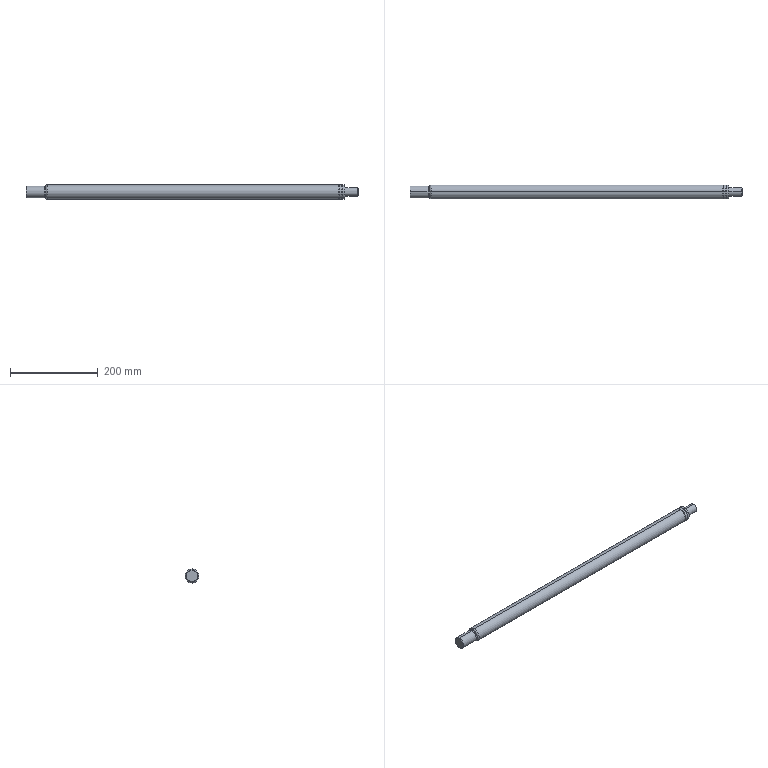Part | SolidWorks | features Revolution 1 | 1 solid | 33 faces | box 755 x 32 x 32 mm | volume 580870 mm3 | cylinder 16 | plane 9 | cone 6 | torus 2 | commonest cylinder face diameters 32 x6 29 x4 20 x2 25 x2 27 x2
STEP:
#1=CARTESIAN_POINT('',(755.,0.,9.));
#2=VERTEX_POINT('',#1);
#3=CARTESIAN_POINT('',(755.,0.,-9.));
#4=VERTEX_POINT('',#3);
#5=CARTESIAN_POINT('',(755.,0.,0.));
#6=DIRECTION('',(-1.,0.,0.));
#7=DIRECTION('',(0.,0.,1.));
#8=AXIS2_PLACEMENT_3D('',#5,#6,#7);
#9=CIRCLE('',#8,9.);
#10=EDGE_CURVE('',#2,#4,#9,.T.);
#11=ORIENTED_EDGE('',*,*,#10,.T.);
#12=CARTESIAN_POINT('',(754.,0.,-10.));
#13=VERTEX_POINT('',#12);
#14=CARTESIAN_POINT('',(755.,0.,-9.));
#15=DIRECTION('',(-0.7071,0.,-0.7071));
#16=VECTOR('',#15,1000.);
#17=LINE('',#14,#16);
#18=EDGE_CURVE('',#4,#13,#17,.T.);
#19=ORIENTED_EDGE('',*,*,#18,.T.);
#20=CARTESIAN_POINT('',(754.,0.,10.));
#21=VERTEX_POINT('',#20);
#22=CARTESIAN_POINT('',(754.,0.,0.));
#23=DIRECTION('',(-1.,0.,0.));
#24=DIRECTION('',(0.,0.,1.));
#25=AXIS2_PLACEMENT_3D('',#22,#23,#24);
#26=CIRCLE('',#25,10.);
#27=EDGE_CURVE('',#21,#13,#26,.T.);
#28=ORIENTED_EDGE('',*,*,#27,.F.);
#29=CARTESIAN_POINT('',(755.,0.,9.));
#30=DIRECTION('',(-0.7071,0.,0.7071));
#31=VECTOR('',#30,1000.);
#32=LINE('',#29,#31);
#33=EDGE_CURVE('',#2,#21,#32,.T.);
#34=ORIENTED_EDGE('',*,*,#33,.F.);
#35=EDGE_LOOP('',(#11,#19,#28,#34));
#36=FACE_OUTER_BOUND('',#35,.T.);
#37=CARTESIAN_POINT('',(755.,0.,0.));
#38=DIRECTION('',(-1.,0.,0.));
#39=DIRECTION('',(0.,0.,1.));
#40=AXIS2_PLACEMENT_3D('',#37,#38,#39);
#41=CONICAL_SURFACE('',#40,9.,0.7854);
#42=ADVANCED_FACE('',(#36),#41,.T.);
#43=ORIENTED_EDGE('',*,*,#27,.T.);
#44=CARTESIAN_POINT('',(725.,0.,-10.));
#45=VERTEX_POINT('',#44);
#46=CARTESIAN_POINT('',(0.,0.,-10.));
#47=DIRECTION('',(-1.,0.,0.));
#48=VECTOR('',#47,1000.);
#49=LINE('',#46,#48);
#50=EDGE_CURVE('',#13,#45,#49,.T.);
#51=ORIENTED_EDGE('',*,*,#50,.T.);
#52=CARTESIAN_POINT('',(725.,0.,10.));
#53=VERTEX_POINT('',#52);
#54=CARTESIAN_POINT('',(725.,0.,0.));
#55=DIRECTION('',(-1.,0.,0.));
#56=DIRECTION('',(0.,0.,1.));
#57=AXIS2_PLACEMENT_3D('',#54,#55,#56);
#58=CIRCLE('',#57,10.);
#59=EDGE_CURVE('',#53,#45,#58,.T.);
#60=ORIENTED_EDGE('',*,*,#59,.F.);
#61=CARTESIAN_POINT('',(0.,0.,10.));
#62=DIRECTION('',(-1.,0.,0.));
#63=VECTOR('',#62,1000.);
#64=LINE('',#61,#63);
#65=EDGE_CURVE('',#21,#53,#64,.T.);
#66=ORIENTED_EDGE('',*,*,#65,.F.);
#67=EDGE_LOOP('',(#43,#51,#60,#66));
#68=FACE_OUTER_BOUND('',#67,.T.);
#69=CARTESIAN_POINT('',(0.,0.,0.));
#70=DIRECTION('',(-1.,0.,0.));
#71=DIRECTION('',(0.,0.,1.));
#72=AXIS2_PLACEMENT_3D('',#69,#70,#71);
#73=CYLINDRICAL_SURFACE('',#72,10.);
#74=ADVANCED_FACE('',(#68),#73,.T.);
#75=CARTESIAN_POINT('',(725.,0.,15.));
#76=VERTEX_POINT('',#75);
#77=CARTESIAN_POINT('',(725.,0.,-15.));
#78=VERTEX_POINT('',#77);
#79=CARTESIAN_POINT('',(725.,0.,0.));
#80=DIRECTION('',(-1.,0.,0.));
#81=DIRECTION('',(0.,0.,1.));
#82=AXIS2_PLACEMENT_3D('',#79,#80,#81);
#83=CIRCLE('',#82,15.);
#84=EDGE_CURVE('',#76,#78,#83,.T.);
#85=ORIENTED_EDGE('',*,*,#84,.T.);
#86=CARTESIAN_POINT('',(724.,0.,-16.));
#87=VERTEX_POINT('',#86);
#88=CARTESIAN_POINT('',(725.,0.,-15.));
#89=DIRECTION('',(-0.7071,0.,-0.7071));
#90=VECTOR('',#89,1000.);
#91=LINE('',#88,#90);
#92=EDGE_CURVE('',#78,#87,#91,.T.);
#93=ORIENTED_EDGE('',*,*,#92,.T.);
#94=CARTESIAN_POINT('',(724.,0.,16.));
#95=VERTEX_POINT('',#94);
#96=CARTESIAN_POINT('',(724.,0.,0.));
#97=DIRECTION('',(-1.,0.,0.));
#98=DIRECTION('',(0.,0.,1.));
#99=AXIS2_PLACEMENT_3D('',#96,#97,#98);
#100=CIRCLE('',#99,16.);
#101=EDGE_CURVE('',#95,#87,#100,.T.);
#102=ORIENTED_EDGE('',*,*,#101,.F.);
#103=CARTESIAN_POINT('',(725.,0.,15.));
#104=DIRECTION('',(-0.7071,0.,0.7071));
#105=VECTOR('',#104,1000.);
#106=LINE('',#103,#105);
#107=EDGE_CURVE('',#76,#95,#106,.T.);
#108=ORIENTED_EDGE('',*,*,#107,.F.);
#109=EDGE_LOOP('',(#85,#93,#102,#108));
#110=FACE_OUTER_BOUND('',#109,.T.);
#111=CARTESIAN_POINT('',(725.,0.,0.));
#112=DIRECTION('',(-1.,0.,0.));
#113=DIRECTION('',(0.,0.,1.));
#114=AXIS2_PLACEMENT_3D('',#111,#112,#113);
#115=CONICAL_SURFACE('',#114,15.,0.7854);
#116=ADVANCED_FACE('',(#110),#115,.T.);
#117=ORIENTED_EDGE('',*,*,#101,.T.);
#118=CARTESIAN_POINT('',(720.,0.,-16.));
#119=VERTEX_POINT('',#118);
#120=CARTESIAN_POINT('',(0.,0.,-16.));
#121=DIRECTION('',(-1.,0.,0.));
#122=VECTOR('',#121,1000.);
#123=LINE('',#120,#122);
#124=EDGE_CURVE('',#87,#119,#123,.T.);
#125=ORIENTED_EDGE('',*,*,#124,.T.);
#126=CARTESIAN_POINT('',(720.,0.,16.));
#127=VERTEX_POINT('',#126);
#128=CARTESIAN_POINT('',(720.,0.,0.));
#129=DIRECTION('',(-1.,0.,0.));
#130=DIRECTION('',(0.,0.,1.));
#131=AXIS2_PLACEMENT_3D('',#128,#129,#130);
#132=CIRCLE('',#131,16.);
#133=EDGE_CURVE('',#127,#119,#132,.T.);
#134=ORIENTED_EDGE('',*,*,#133,.F.);
#135=CARTESIAN_POINT('',(0.,0.,16.));
#136=DIRECTION('',(-1.,0.,0.));
#137=VECTOR('',#136,1000.);
#138=LINE('',#135,#137);
#139=EDGE_CURVE('',#95,#127,#138,.T.);
#140=ORIENTED_EDGE('',*,*,#139,.F.);
#141=EDGE_LOOP('',(#117,#125,#134,#140));
#142=FACE_OUTER_BOUND('',#141,.T.);
#143=CARTESIAN_POINT('',(0.,0.,0.));
#144=DIRECTION('',(-1.,0.,0.));
#145=DIRECTION('',(0.,0.,1.));
#146=AXIS2_PLACEMENT_3D('',#143,#144,#145);
#147=CYLINDRICAL_SURFACE('',#146,16.);
#148=ADVANCED_FACE('',(#142),#147,.T.);
#149=CARTESIAN_POINT('',(720.,0.,14.5));
#150=VERTEX_POINT('',#149);
#151=CARTESIAN_POINT('',(720.,0.,-14.5));
#152=VERTEX_POINT('',#151);
#153=CARTESIAN_POINT('',(720.,0.,0.));
#154=DIRECTION('',(-1.,0.,0.));
#155=DIRECTION('',(0.,0.,1.));
#156=AXIS2_PLACEMENT_3D('',#153,#154,#155);
#157=CIRCLE('',#156,14.5);
#158=EDGE_CURVE('',#150,#152,#157,.T.);
#159=ORIENTED_EDGE('',*,*,#158,.T.);
#160=CARTESIAN_POINT('',(718.,0.,-14.5));
#161=VERTEX_POINT('',#160);
#162=CARTESIAN_POINT('',(0.,0.,-14.5));
#163=DIRECTION('',(-1.,0.,0.));
#164=VECTOR('',#163,1000.);
#165=LINE('',#162,#164);
#166=EDGE_CURVE('',#152,#161,#165,.T.);
#167=ORIENTED_EDGE('',*,*,#166,.T.);
#168=CARTESIAN_POINT('',(718.,0.,14.5));
#169=VERTEX_POINT('',#168);
#170=CARTESIAN_POINT('',(718.,0.,0.));
#171=DIRECTION('',(-1.,0.,0.));
#172=DIRECTION('',(0.,0.,1.));
#173=AXIS2_PLACEMENT_3D('',#170,#171,#172);
#174=CIRCLE('',#173,14.5);
#175=EDGE_CURVE('',#169,#161,#174,.T.);
#176=ORIENTED_EDGE('',*,*,#175,.F.);
#177=CARTESIAN_POINT('',(0.,0.,14.5));
#178=DIRECTION('',(-1.,0.,0.));
#179=VECTOR('',#178,1000.);
#180=LINE('',#177,#179);
#181=EDGE_CURVE('',#150,#169,#180,.T.);
#182=ORIENTED_EDGE('',*,*,#181,.F.);
#183=EDGE_LOOP('',(#159,#167,#176,#182));
#184=FACE_OUTER_BOUND('',#183,.T.);
#185=CARTESIAN_POINT('',(0.,0.,0.));
#186=DIRECTION('',(-1.,0.,0.));
#187=DIRECTION('',(0.,0.,1.));
#188=AXIS2_PLACEMENT_3D('',#185,#186,#187);
#189=CYLINDRICAL_SURFACE('',#188,14.5);
#190=ADVANCED_FACE('',(#184),#189,.T.);
#191=CARTESIAN_POINT('',(718.,0.,16.));
#192=VERTEX_POINT('',#191);
#193=CARTESIAN_POINT('',(718.,0.,-16.));
#194=VERTEX_POINT('',#193);
#195=CARTESIAN_POINT('',(718.,0.,0.));
#196=DIRECTION('',(-1.,0.,0.));
#197=DIRECTION('',(0.,0.,1.));
#198=AXIS2_PLACEMENT_3D('',#195,#196,#197);
#199=CIRCLE('',#198,16.);
#200=EDGE_CURVE('',#192,#194,#199,.T.);
#201=ORIENTED_EDGE('',*,*,#200,.T.);
#202=CARTESIAN_POINT('',(713.,0.,-16.));
#203=VERTEX_POINT('',#202);
#204=CARTESIAN_POINT('',(0.,0.,-16.));
#205=DIRECTION('',(-1.,0.,0.));
#206=VECTOR('',#205,1000.);
#207=LINE('',#204,#206);
#208=EDGE_CURVE('',#194,#203,#207,.T.);
#209=ORIENTED_EDGE('',*,*,#208,.T.);
#210=CARTESIAN_POINT('',(713.,0.,16.));
#211=VERTEX_POINT('',#210);
#212=CARTESIAN_POINT('',(713.,0.,0.));
#213=DIRECTION('',(-1.,0.,0.));
#214=DIRECTION('',(0.,0.,1.));
#215=AXIS2_PLACEMENT_3D('',#212,#213,#214);
#216=CIRCLE('',#215,16.);
#217=EDGE_CURVE('',#211,#203,#216,.T.);
#218=ORIENTED_EDGE('',*,*,#217,.F.);
#219=CARTESIAN_POINT('',(0.,0.,16.));
#220=DIRECTION('',(-1.,0.,0.));
#221=VECTOR('',#220,1000.);
#222=LINE('',#219,#221);
#223=EDGE_CURVE('',#192,#211,#222,.T.);
#224=ORIENTED_EDGE('',*,*,#223,.F.);
#225=EDGE_LOOP('',(#201,#209,#218,#224));
#226=FACE_OUTER_BOUND('',#225,.T.);
#227=CARTESIAN_POINT('',(0.,0.,0.));
#228=DIRECTION('',(-1.,0.,0.));
#229=DIRECTION('',(0.,0.,1.));
#230=AXIS2_PLACEMENT_3D('',#227,#228,#229);
#231=CYLINDRICAL_SURFACE('',#230,16.);
#232=ADVANCED_FACE('',(#226),#231,.T.);
#233=CARTESIAN_POINT('',(713.,0.,14.5));
#234=VERTEX_POINT('',#233);
#235=CARTESIAN_POINT('',(713.,0.,-14.5));
#236=VERTEX_POINT('',#235);
#237=CARTESIAN_POINT('',(713.,0.,0.));
#238=DIRECTION('',(-1.,0.,0.));
#239=DIRECTION('',(0.,0.,1.));
#240=AXIS2_PLACEMENT_3D('',#237,#238,#239);
#241=CIRCLE('',#240,14.5);
#242=EDGE_CURVE('',#234,#236,#241,.T.);
#243=ORIENTED_EDGE('',*,*,#242,.T.);
#244=CARTESIAN_POINT('',(711.,0.,-14.5));
#245=VERTEX_POINT('',#244);
#246=CARTESIAN_POINT('',(0.,0.,-14.5));
#247=DIRECTION('',(-1.,0.,0.));
#248=VECTOR('',#247,1000.);
#249=LINE('',#246,#248);
#250=EDGE_CURVE('',#236,#245,#249,.T.);
#251=ORIENTED_EDGE('',*,*,#250,.T.);
#252=CARTESIAN_POINT('',(711.,0.,14.5));
#253=VERTEX_POINT('',#252);
#254=CARTESIAN_POINT('',(711.,0.,0.));
#255=DIRECTION('',(-1.,0.,0.));
#256=DIRECTION('',(0.,0.,1.));
#257=AXIS2_PLACEMENT_3D('',#254,#255,#256);
#258=CIRCLE('',#257,14.5);
#259=EDGE_CURVE('',#253,#245,#258,.T.);
#260=ORIENTED_EDGE('',*,*,#259,.F.);
#261=CARTESIAN_POINT('',(0.,0.,14.5));
#262=DIRECTION('',(-1.,0.,0.));
#263=VECTOR('',#262,1000.);
#264=LINE('',#261,#263);
#265=EDGE_CURVE('',#234,#253,#264,.T.);
#266=ORIENTED_EDGE('',*,*,#265,.F.);
#267=EDGE_LOOP('',(#243,#251,#260,#266));
#268=FACE_OUTER_BOUND('',#267,.T.);
#269=CARTESIAN_POINT('',(0.,0.,0.));
#270=DIRECTION('',(-1.,0.,0.));
#271=DIRECTION('',(0.,0.,1.));
#272=AXIS2_PLACEMENT_3D('',#269,#270,#271);
#273=CYLINDRICAL_SURFACE('',#272,14.5);
#274=ADVANCED_FACE('',(#268),#273,.T.);
#275=CARTESIAN_POINT('',(711.,0.,16.));
#276=VERTEX_POINT('',#275);
#277=CARTESIAN_POINT('',(711.,0.,-16.));
#278=VERTEX_POINT('',#277);
#279=CARTESIAN_POINT('',(711.,0.,0.));
#280=DIRECTION('',(-1.,0.,0.));
#281=DIRECTION('',(0.,0.,1.));
#282=AXIS2_PLACEMENT_3D('',#279,#280,#281);
#283=CIRCLE('',#282,16.);
#284=EDGE_CURVE('',#276,#278,#283,.T.);
#285=ORIENTED_EDGE('',*,*,#284,.T.);
#286=CARTESIAN_POINT('',(48.,0.,-16.));
#287=VERTEX_POINT('',#286);
#288=CARTESIAN_POINT('',(0.,0.,-16.));
#289=DIRECTION('',(-1.,0.,0.));
#290=VECTOR('',#289,1000.);
#291=LINE('',#288,#290);
#292=EDGE_CURVE('',#278,#287,#291,.T.);
#293=ORIENTED_EDGE('',*,*,#292,.T.);
#294=CARTESIAN_POINT('',(48.,0.,16.));
#295=VERTEX_POINT('',#294);
#296=CARTESIAN_POINT('',(48.,0.,0.));
#297=DIRECTION('',(-1.,0.,0.));
#298=DIRECTION('',(0.,0.,1.));
#299=AXIS2_PLACEMENT_3D('',#296,#297,#298);
#300=CIRCLE('',#299,16.);
#301=EDGE_CURVE('',#295,#287,#300,.T.);
#302=ORIENTED_EDGE('',*,*,#301,.F.);
#303=CARTESIAN_POINT('',(0.,0.,16.));
#304=DIRECTION('',(-1.,0.,0.));
#305=VECTOR('',#304,1000.);
#306=LINE('',#303,#305);
#307=EDGE_CURVE('',#276,#295,#306,.T.);
#308=ORIENTED_EDGE('',*,*,#307,.F.);
#309=EDGE_LOOP('',(#285,#293,#302,#308));
#310=FACE_OUTER_BOUND('',#309,.T.);
#311=CARTESIAN_POINT('',(0.,0.,0.));
#312=DIRECTION('',(-1.,0.,0.));
#313=DIRECTION('',(0.,0.,1.));
#314=AXIS2_PLACEMENT_3D('',#311,#312,#313);
#315=CYLINDRICAL_SURFACE('',#314,16.);
#316=ADVANCED_FACE('',(#310),#315,.T.);
#317=ORIENTED_EDGE('',*,*,#301,.T.);
#318=CARTESIAN_POINT('',(45.,0.,-13.));
#319=VERTEX_POINT('',#318);
#320=CARTESIAN_POINT('',(48.,0.,-13.));
#321=DIRECTION('',(0.,1.,0.));
#322=DIRECTION('',(0.,0.,1.));
#323=AXIS2_PLACEMENT_3D('',#320,#321,#322);
#324=CIRCLE('',#323,3.);
#325=EDGE_CURVE('',#287,#319,#324,.T.);
#326=ORIENTED_EDGE('',*,*,#325,.T.);
#327=CARTESIAN_POINT('',(45.,0.,13.));
#328=VERTEX_POINT('',#327);
#329=CARTESIAN_POINT('',(45.,0.,0.));
#330=DIRECTION('',(-1.,0.,0.));
#331=DIRECTION('',(0.,0.,1.));
#332=AXIS2_PLACEMENT_3D('',#329,#330,#331);
#333=CIRCLE('',#332,13.);
#334=EDGE_CURVE('',#328,#319,#333,.T.);
#335=ORIENTED_EDGE('',*,*,#334,.F.);
#336=CARTESIAN_POINT('',(48.,0.,13.));
#337=DIRECTION('',(0.,-1.,0.));
#338=DIRECTION('',(0.,0.,-1.));
#339=AXIS2_PLACEMENT_3D('',#336,#337,#338);
#340=CIRCLE('',#339,3.);
#341=EDGE_CURVE('',#295,#328,#340,.T.);
#342=ORIENTED_EDGE('',*,*,#341,.F.);
#343=EDGE_LOOP('',(#317,#326,#335,#342));
#344=FACE_OUTER_BOUND('',#343,.T.);
#345=CARTESIAN_POINT('',(48.,0.,0.));
#346=DIRECTION('',(-1.,0.,0.));
#347=DIRECTION('',(0.,0.,1.));
#348=AXIS2_PLACEMENT_3D('',#345,#346,#347);
#349=TOROIDAL_SURFACE('',#348,13.,3.);
#350=ADVANCED_FACE('',(#344),#349,.T.);
#351=CARTESIAN_POINT('',(45.,0.,12.5));
#352=VERTEX_POINT('',#351);
#353=CARTESIAN_POINT('',(45.,0.,-12.5));
#354=VERTEX_POINT('',#353);
#355=CARTESIAN_POINT('',(45.,0.,0.));
#356=DIRECTION('',(-1.,0.,0.));
#357=DIRECTION('',(0.,0.,1.));
#358=AXIS2_PLACEMENT_3D('',#355,#356,#357);
#359=CIRCLE('',#358,12.5);
#360=EDGE_CURVE('',#352,#354,#359,.T.);
#361=ORIENTED_EDGE('',*,*,#360,.T.);
#362=CARTESIAN_POINT('',(41.,0.,-12.5));
#363=VERTEX_POINT('',#362);
#364=CARTESIAN_POINT('',(0.,0.,-12.5));
#365=DIRECTION('',(-1.,0.,0.));
#366=VECTOR('',#365,1000.);
#367=LINE('',#364,#366);
#368=EDGE_CURVE('',#354,#363,#367,.T.);
#369=ORIENTED_EDGE('',*,*,#368,.T.);
#370=CARTESIAN_POINT('',(41.,0.,12.5));
#371=VERTEX_POINT('',#370);
#372=CARTESIAN_POINT('',(41.,0.,0.));
#373=DIRECTION('',(-1.,0.,0.));
#374=DIRECTION('',(0.,0.,1.));
#375=AXIS2_PLACEMENT_3D('',#372,#373,#374);
#376=CIRCLE('',#375,12.5);
#377=EDGE_CURVE('',#371,#363,#376,.T.);
#378=ORIENTED_EDGE('',*,*,#377,.F.);
#379=CARTESIAN_POINT('',(0.,0.,12.5));
#380=DIRECTION('',(-1.,0.,0.));
#381=VECTOR('',#380,1000.);
#382=LINE('',#379,#381);
#383=EDGE_CURVE('',#352,#371,#382,.T.);
#384=ORIENTED_EDGE('',*,*,#383,.F.);
#385=EDGE_LOOP('',(#361,#369,#378,#384));
#386=FACE_OUTER_BOUND('',#385,.T.);
#387=CARTESIAN_POINT('',(0.,0.,0.));
#388=DIRECTION('',(-1.,0.,0.));
#389=DIRECTION('',(0.,0.,1.));
#390=AXIS2_PLACEMENT_3D('',#387,#388,#389);
#391=CYLINDRICAL_SURFACE('',#390,12.5);
#392=ADVANCED_FACE('',(#386),#391,.T.);
#393=CARTESIAN_POINT('',(41.,0.,13.5));
#394=VERTEX_POINT('',#393);
#395=CARTESIAN_POINT('',(41.,0.,-13.5));
#396=VERTEX_POINT('',#395);
#397=CARTESIAN_POINT('',(41.,0.,0.));
#398=DIRECTION('',(-1.,0.,0.));
#399=DIRECTION('',(0.,0.,1.));
#400=AXIS2_PLACEMENT_3D('',#397,#398,#399);
#401=CIRCLE('',#400,13.5);
#402=EDGE_CURVE('',#394,#396,#401,.T.);
#403=ORIENTED_EDGE('',*,*,#402,.T.);
#404=CARTESIAN_POINT('',(1.,0.,-13.5));
#405=VERTEX_POINT('',#404);
#406=CARTESIAN_POINT('',(0.,0.,-13.5));
#407=DIRECTION('',(-1.,0.,0.));
#408=VECTOR('',#407,1000.);
#409=LINE('',#406,#408);
#410=EDGE_CURVE('',#396,#405,#409,.T.);
#411=ORIENTED_EDGE('',*,*,#410,.T.);
#412=CARTESIAN_POINT('',(1.,0.,13.5));
#413=VERTEX_POINT('',#412);
#414=CARTESIAN_POINT('',(1.,0.,0.));
#415=DIRECTION('',(-1.,0.,0.));
#416=DIRECTION('',(0.,0.,1.));
#417=AXIS2_PLACEMENT_3D('',#414,#415,#416);
#418=CIRCLE('',#417,13.5);
#419=EDGE_CURVE('',#413,#405,#418,.T.);
#420=ORIENTED_EDGE('',*,*,#419,.F.);
#421=CARTESIAN_POINT('',(0.,0.,13.5));
#422=DIRECTION('',(-1.,0.,0.));
#423=VECTOR('',#422,1000.);
#424=LINE('',#421,#423);
#425=EDGE_CURVE('',#394,#413,#424,.T.);
#426=ORIENTED_EDGE('',*,*,#425,.F.);
#427=EDGE_LOOP('',(#403,#411,#420,#426));
#428=FACE_OUTER_BOUND('',#427,.T.);
#429=CARTESIAN_POINT('',(0.,0.,0.));
#430=DIRECTION('',(-1.,0.,0.));
#431=DIRECTION('',(0.,0.,1.));
#432=AXIS2_PLACEMENT_3D('',#429,#430,#431);
#433=CYLINDRICAL_SURFACE('',#432,13.5);
#434=ADVANCED_FACE('',(#428),#433,.T.);
#435=CARTESIAN_POINT('',(0.,0.,12.5));
#436=VERTEX_POINT('',#435);
#437=CARTESIAN_POINT('',(0.,0.,-12.5));
#438=VERTEX_POINT('',#437);
#439=CARTESIAN_POINT('',(0.,0.,0.));
#440=DIRECTION('',(-1.,0.,0.));
#441=DIRECTION('',(0.,0.,1.));
#442=AXIS2_PLACEMENT_3D('',#439,#440,#441);
#443=CIRCLE('',#442,12.5);
#444=EDGE_CURVE('',#436,#438,#443,.T.);
#445=ORIENTED_EDGE('',*,*,#444,.F.);
#446=CARTESIAN_POINT('',(1.,0.,13.5));
#447=DIRECTION('',(0.7071,0.,0.7071));
#448=VECTOR('',#447,1000.);
#449=LINE('',#446,#448);
#450=EDGE_CURVE('',#436,#413,#449,.T.);
#451=ORIENTED_EDGE('',*,*,#450,.T.);
#452=ORIENTED_EDGE('',*,*,#419,.T.);
#453=CARTESIAN_POINT('',(1.,0.,-13.5));
#454=DIRECTION('',(0.7071,0.,-0.7071));
#455=VECTOR('',#454,1000.);
#456=LINE('',#453,#455);
#457=EDGE_CURVE('',#438,#405,#456,.T.);
#458=ORIENTED_EDGE('',*,*,#457,.F.);
#459=EDGE_LOOP('',(#445,#451,#452,#458));
#460=FACE_OUTER_BOUND('',#459,.T.);
#461=CARTESIAN_POINT('',(1.,0.,0.));
#462=DIRECTION('',(1.,0.,0.));
#463=DIRECTION('',(0.,0.,-1.));
#464=AXIS2_PLACEMENT_3D('',#461,#462,#463);
#465=CONICAL_SURFACE('',#464,13.5,0.7854);
#466=ADVANCED_FACE('',(#460),#465,.T.);
#467=CARTESIAN_POINT('',(0.,0.,0.));
#468=DIRECTION('',(-1.,0.,0.));
#469=DIRECTION('',(0.,0.,1.));
#470=AXIS2_PLACEMENT_3D('',#467,#468,#469);
#471=CIRCLE('',#470,12.5);
#472=EDGE_CURVE('',#438,#436,#471,.T.);
#473=ORIENTED_EDGE('',*,*,#472,.T.);
#474=ORIENTED_EDGE('',*,*,#444,.T.);
#475=EDGE_LOOP('',(#473,#474));
#476=FACE_OUTER_BOUND('',#475,.T.);
#477=CARTESIAN_POINT('',(0.,0.,0.));
#478=DIRECTION('',(1.,0.,0.));
#479=DIRECTION('',(0.,0.,-1.));
#480=AXIS2_PLACEMENT_3D('',#477,#478,#479);
#481=PLANE('',#480);
#482=ADVANCED_FACE('',(#476),#481,.F.);
#483=ORIENTED_EDGE('',*,*,#450,.F.);
#484=ORIENTED_EDGE('',*,*,#472,.F.);
#485=ORIENTED_EDGE('',*,*,#457,.T.);
#486=CARTESIAN_POINT('',(1.,0.,0.));
#487=DIRECTION('',(-1.,0.,0.));
#488=DIRECTION('',(0.,0.,1.));
#489=AXIS2_PLACEMENT_3D('',#486,#487,#488);
#490=CIRCLE('',#489,13.5);
#491=EDGE_CURVE('',#405,#413,#490,.T.);
#492=ORIENTED_EDGE('',*,*,#491,.T.);
#493=EDGE_LOOP('',(#483,#484,#485,#492));
#494=FACE_OUTER_BOUND('',#493,.T.);
#495=CARTESIAN_POINT('',(1.,0.,0.));
#496=DIRECTION('',(1.,0.,0.));
#497=DIRECTION('',(0.,0.,-1.));
#498=AXIS2_PLACEMENT_3D('',#495,#496,#497);
#499=CONICAL_SURFACE('',#498,13.5,0.7854);
#500=ADVANCED_FACE('',(#494),#499,.T.);
#501=ORIENTED_EDGE('',*,*,#410,.F.);
#502=CARTESIAN_POINT('',(41.,0.,0.));
#503=DIRECTION('',(-1.,0.,0.));
#504=DIRECTION('',(0.,0.,1.));
#505=AXIS2_PLACEMENT_3D('',#502,#503,#504);
#506=CIRCLE('',#505,13.5);
#507=EDGE_CURVE('',#396,#394,#506,.T.);
#508=ORIENTED_EDGE('',*,*,#507,.T.);
#509=ORIENTED_EDGE('',*,*,#425,.T.);
#510=ORIENTED_EDGE('',*,*,#491,.F.);
#511=EDGE_LOOP('',(#501,#508,#509,#510));
#512=FACE_OUTER_BOUND('',#511,.T.);
#513=CARTESIAN_POINT('',(0.,0.,0.));
#514=DIRECTION('',(-1.,0.,0.));
#515=DIRECTION('',(0.,0.,1.));
#516=AXIS2_PLACEMENT_3D('',#513,#514,#515);
#517=CYLINDRICAL_SURFACE('',#516,13.5);
#518=ADVANCED_FACE('',(#512),#517,.T.);
#519=ORIENTED_EDGE('',*,*,#402,.F.);
#520=ORIENTED_EDGE('',*,*,#507,.F.);
#521=EDGE_LOOP('',(#519,#520));
#522=FACE_OUTER_BOUND('',#521,.T.);
#523=ORIENTED_EDGE('',*,*,#377,.T.);
#524=CARTESIAN_POINT('',(41.,0.,0.));
#525=DIRECTION('',(-1.,0.,0.));
#526=DIRECTION('',(0.,0.,1.));
#527=AXIS2_PLACEMENT_3D('',#524,#525,#526);
#528=CIRCLE('',#527,12.5);
#529=EDGE_CURVE('',#363,#371,#528,.T.);
#530=ORIENTED_EDGE('',*,*,#529,.T.);
#531=EDGE_LOOP('',(#523,#530));
#532=FACE_BOUND('',#531,.T.);
#533=CARTESIAN_POINT('',(41.,13.5,0.));
#534=DIRECTION('',(-1.,0.,0.));
#535=DIRECTION('',(0.,0.,1.));
#536=AXIS2_PLACEMENT_3D('',#533,#534,#535);
#537=PLANE('',#536);
#538=ADVANCED_FACE('',(#522,#532),#537,.F.);
#539=ORIENTED_EDGE('',*,*,#368,.F.);
#540=CARTESIAN_POINT('',(45.,0.,0.));
#541=DIRECTION('',(-1.,0.,0.));
#542=DIRECTION('',(0.,0.,1.));
#543=AXIS2_PLACEMENT_3D('',#540,#541,#542);
#544=CIRCLE('',#543,12.5);
#545=EDGE_CURVE('',#354,#352,#544,.T.);
#546=ORIENTED_EDGE('',*,*,#545,.T.);
#547=ORIENTED_EDGE('',*,*,#383,.T.);
#548=ORIENTED_EDGE('',*,*,#529,.F.);
#549=EDGE_LOOP('',(#539,#546,#547,#548));
#550=FACE_OUTER_BOUND('',#549,.T.);
#551=CARTESIAN_POINT('',(0.,0.,0.));
#552=DIRECTION('',(-1.,0.,0.));
#553=DIRECTION('',(0.,0.,1.));
#554=AXIS2_PLACEMENT_3D('',#551,#552,#553);
#555=CYLINDRICAL_SURFACE('',#554,12.5);
#556=ADVANCED_FACE('',(#550),#555,.T.);
#557=ORIENTED_EDGE('',*,*,#360,.F.);
#558=ORIENTED_EDGE('',*,*,#545,.F.);
#559=EDGE_LOOP('',(#557,#558));
#560=FACE_BOUND('',#559,.T.);
#561=ORIENTED_EDGE('',*,*,#334,.T.);
#562=CARTESIAN_POINT('',(45.,0.,0.));
#563=DIRECTION('',(-1.,0.,0.));
#564=DIRECTION('',(0.,0.,1.));
#565=AXIS2_PLACEMENT_3D('',#562,#563,#564);
#566=CIRCLE('',#565,13.);
#567=EDGE_CURVE('',#319,#328,#566,.T.);
#568=ORIENTED_EDGE('',*,*,#567,.T.);
#569=EDGE_LOOP('',(#561,#568));
#570=FACE_OUTER_BOUND('',#569,.T.);
#571=CARTESIAN_POINT('',(45.,12.5,0.));
#572=DIRECTION('',(1.,0.,0.));
#573=DIRECTION('',(0.,0.,-1.));
#574=AXIS2_PLACEMENT_3D('',#571,#572,#573);
#575=PLANE('',#574);
#576=ADVANCED_FACE('',(#560,#570),#575,.F.);
#577=ORIENTED_EDGE('',*,*,#325,.F.);
#578=CARTESIAN_POINT('',(48.,0.,0.));
#579=DIRECTION('',(-1.,0.,0.));
#580=DIRECTION('',(0.,0.,1.));
#581=AXIS2_PLACEMENT_3D('',#578,#579,#580);
#582=CIRCLE('',#581,16.);
#583=EDGE_CURVE('',#287,#295,#582,.T.);
#584=ORIENTED_EDGE('',*,*,#583,.T.);
#585=ORIENTED_EDGE('',*,*,#341,.T.);
#586=ORIENTED_EDGE('',*,*,#567,.F.);
#587=EDGE_LOOP('',(#577,#584,#585,#586));
#588=FACE_OUTER_BOUND('',#587,.T.);
#589=CARTESIAN_POINT('',(48.,0.,0.));
#590=DIRECTION('',(-1.,0.,0.));
#591=DIRECTION('',(0.,0.,1.));
#592=AXIS2_PLACEMENT_3D('',#589,#590,#591);
#593=TOROIDAL_SURFACE('',#592,13.,3.);
#594=ADVANCED_FACE('',(#588),#593,.T.);
#595=ORIENTED_EDGE('',*,*,#292,.F.);
#596=CARTESIAN_POINT('',(711.,0.,0.));
#597=DIRECTION('',(-1.,0.,0.));
#598=DIRECTION('',(0.,0.,1.));
#599=AXIS2_PLACEMENT_3D('',#596,#597,#598);
#600=CIRCLE('',#599,16.);
#601=EDGE_CURVE('',#278,#276,#600,.T.);
#602=ORIENTED_EDGE('',*,*,#601,.T.);
#603=ORIENTED_EDGE('',*,*,#307,.T.);
#604=ORIENTED_EDGE('',*,*,#583,.F.);
#605=EDGE_LOOP('',(#595,#602,#603,#604));
#606=FACE_OUTER_BOUND('',#605,.T.);
#607=CARTESIAN_POINT('',(0.,0.,0.));
#608=DIRECTION('',(-1.,0.,0.));
#609=DIRECTION('',(0.,0.,1.));
#610=AXIS2_PLACEMENT_3D('',#607,#608,#609);
#611=CYLINDRICAL_SURFACE('',#610,16.);
#612=ADVANCED_FACE('',(#606),#611,.T.);
#613=ORIENTED_EDGE('',*,*,#284,.F.);
#614=ORIENTED_EDGE('',*,*,#601,.F.);
#615=EDGE_LOOP('',(#613,#614));
#616=FACE_OUTER_BOUND('',#615,.T.);
#617=ORIENTED_EDGE('',*,*,#259,.T.);
#618=CARTESIAN_POINT('',(711.,0.,0.));
#619=DIRECTION('',(-1.,0.,0.));
#620=DIRECTION('',(0.,0.,1.));
#621=AXIS2_PLACEMENT_3D('',#618,#619,#620);
#622=CIRCLE('',#621,14.5);
#623=EDGE_CURVE('',#245,#253,#622,.T.);
#624=ORIENTED_EDGE('',*,*,#623,.T.);
#625=EDGE_LOOP('',(#617,#624));
#626=FACE_BOUND('',#625,.T.);
#627=CARTESIAN_POINT('',(711.,16.,0.));
#628=DIRECTION('',(-1.,0.,0.));
#629=DIRECTION('',(0.,0.,1.));
#630=AXIS2_PLACEMENT_3D('',#627,#628,#629);
#631=PLANE('',#630);
#632=ADVANCED_FACE('',(#616,#626),#631,.F.);
#633=ORIENTED_EDGE('',*,*,#250,.F.);
#634=CARTESIAN_POINT('',(713.,0.,0.));
#635=DIRECTION('',(-1.,0.,0.));
#636=DIRECTION('',(0.,0.,1.));
#637=AXIS2_PLACEMENT_3D('',#634,#635,#636);
#638=CIRCLE('',#637,14.5);
#639=EDGE_CURVE('',#236,#234,#638,.T.);
#640=ORIENTED_EDGE('',*,*,#639,.T.);
#641=ORIENTED_EDGE('',*,*,#265,.T.);
#642=ORIENTED_EDGE('',*,*,#623,.F.);
#643=EDGE_LOOP('',(#633,#640,#641,#642));
#644=FACE_OUTER_BOUND('',#643,.T.);
#645=CARTESIAN_POINT('',(0.,0.,0.));
#646=DIRECTION('',(-1.,0.,0.));
#647=DIRECTION('',(0.,0.,1.));
#648=AXIS2_PLACEMENT_3D('',#645,#646,#647);
#649=CYLINDRICAL_SURFACE('',#648,14.5);
#650=ADVANCED_FACE('',(#644),#649,.T.);
#651=ORIENTED_EDGE('',*,*,#242,.F.);
#652=ORIENTED_EDGE('',*,*,#639,.F.);
#653=EDGE_LOOP('',(#651,#652));
#654=FACE_BOUND('',#653,.T.);
#655=ORIENTED_EDGE('',*,*,#217,.T.);
#656=CARTESIAN_POINT('',(713.,0.,0.));
#657=DIRECTION('',(-1.,0.,0.));
#658=DIRECTION('',(0.,0.,1.));
#659=AXIS2_PLACEMENT_3D('',#656,#657,#658);
#660=CIRCLE('',#659,16.);
#661=EDGE_CURVE('',#203,#211,#660,.T.);
#662=ORIENTED_EDGE('',*,*,#661,.T.);
#663=EDGE_LOOP('',(#655,#662));
#664=FACE_OUTER_BOUND('',#663,.T.);
#665=CARTESIAN_POINT('',(713.,14.5,0.));
#666=DIRECTION('',(1.,0.,0.));
#667=DIRECTION('',(0.,0.,-1.));
#668=AXIS2_PLACEMENT_3D('',#665,#666,#667);
#669=PLANE('',#668);
#670=ADVANCED_FACE('',(#654,#664),#669,.F.);
#671=ORIENTED_EDGE('',*,*,#208,.F.);
#672=CARTESIAN_POINT('',(718.,0.,0.));
#673=DIRECTION('',(-1.,0.,0.));
#674=DIRECTION('',(0.,0.,1.));
#675=AXIS2_PLACEMENT_3D('',#672,#673,#674);
#676=CIRCLE('',#675,16.);
#677=EDGE_CURVE('',#194,#192,#676,.T.);
#678=ORIENTED_EDGE('',*,*,#677,.T.);
#679=ORIENTED_EDGE('',*,*,#223,.T.);
#680=ORIENTED_EDGE('',*,*,#661,.F.);
#681=EDGE_LOOP('',(#671,#678,#679,#680));
#682=FACE_OUTER_BOUND('',#681,.T.);
#683=CARTESIAN_POINT('',(0.,0.,0.));
#684=DIRECTION('',(-1.,0.,0.));
#685=DIRECTION('',(0.,0.,1.));
#686=AXIS2_PLACEMENT_3D('',#683,#684,#685);
#687=CYLINDRICAL_SURFACE('',#686,16.);
#688=ADVANCED_FACE('',(#682),#687,.T.);
#689=ORIENTED_EDGE('',*,*,#200,.F.);
#690=ORIENTED_EDGE('',*,*,#677,.F.);
#691=EDGE_LOOP('',(#689,#690));
#692=FACE_OUTER_BOUND('',#691,.T.);
#693=ORIENTED_EDGE('',*,*,#175,.T.);
#694=CARTESIAN_POINT('',(718.,0.,0.));
#695=DIRECTION('',(-1.,0.,0.));
#696=DIRECTION('',(0.,0.,1.));
#697=AXIS2_PLACEMENT_3D('',#694,#695,#696);
#698=CIRCLE('',#697,14.5);
#699=EDGE_CURVE('',#161,#169,#698,.T.);
#700=ORIENTED_EDGE('',*,*,#699,.T.);
#701=EDGE_LOOP('',(#693,#700));
#702=FACE_BOUND('',#701,.T.);
#703=CARTESIAN_POINT('',(718.,16.,0.));
#704=DIRECTION('',(-1.,0.,0.));
#705=DIRECTION('',(0.,0.,1.));
#706=AXIS2_PLACEMENT_3D('',#703,#704,#705);
#707=PLANE('',#706);
#708=ADVANCED_FACE('',(#692,#702),#707,.F.);
#709=ORIENTED_EDGE('',*,*,#166,.F.);
#710=CARTESIAN_POINT('',(720.,0.,0.));
#711=DIRECTION('',(-1.,0.,0.));
#712=DIRECTION('',(0.,0.,1.));
#713=AXIS2_PLACEMENT_3D('',#710,#711,#712);
#714=CIRCLE('',#713,14.5);
#715=EDGE_CURVE('',#152,#150,#714,.T.);
#716=ORIENTED_EDGE('',*,*,#715,.T.);
#717=ORIENTED_EDGE('',*,*,#181,.T.);
#718=ORIENTED_EDGE('',*,*,#699,.F.);
#719=EDGE_LOOP('',(#709,#716,#717,#718));
#720=FACE_OUTER_BOUND('',#719,.T.);
#721=CARTESIAN_POINT('',(0.,0.,0.));
#722=DIRECTION('',(-1.,0.,0.));
#723=DIRECTION('',(0.,0.,1.));
#724=AXIS2_PLACEMENT_3D('',#721,#722,#723);
#725=CYLINDRICAL_SURFACE('',#724,14.5);
#726=ADVANCED_FACE('',(#720),#725,.T.);
#727=ORIENTED_EDGE('',*,*,#158,.F.);
#728=ORIENTED_EDGE('',*,*,#715,.F.);
#729=EDGE_LOOP('',(#727,#728));
#730=FACE_BOUND('',#729,.T.);
#731=ORIENTED_EDGE('',*,*,#133,.T.);
#732=CARTESIAN_POINT('',(720.,0.,0.));
#733=DIRECTION('',(-1.,0.,0.));
#734=DIRECTION('',(0.,0.,1.));
#735=AXIS2_PLACEMENT_3D('',#732,#733,#734);
#736=CIRCLE('',#735,16.);
#737=EDGE_CURVE('',#119,#127,#736,.T.);
#738=ORIENTED_EDGE('',*,*,#737,.T.);
#739=EDGE_LOOP('',(#731,#738));
#740=FACE_OUTER_BOUND('',#739,.T.);
#741=CARTESIAN_POINT('',(720.,14.5,0.));
#742=DIRECTION('',(1.,0.,0.));
#743=DIRECTION('',(0.,0.,-1.));
#744=AXIS2_PLACEMENT_3D('',#741,#742,#743);
#745=PLANE('',#744);
#746=ADVANCED_FACE('',(#730,#740),#745,.F.);
#747=ORIENTED_EDGE('',*,*,#124,.F.);
#748=CARTESIAN_POINT('',(724.,0.,0.));
#749=DIRECTION('',(-1.,0.,0.));
#750=DIRECTION('',(0.,0.,1.));
#751=AXIS2_PLACEMENT_3D('',#748,#749,#750);
#752=CIRCLE('',#751,16.);
#753=EDGE_CURVE('',#87,#95,#752,.T.);
#754=ORIENTED_EDGE('',*,*,#753,.T.);
#755=ORIENTED_EDGE('',*,*,#139,.T.);
#756=ORIENTED_EDGE('',*,*,#737,.F.);
#757=EDGE_LOOP('',(#747,#754,#755,#756));
#758=FACE_OUTER_BOUND('',#757,.T.);
#759=CARTESIAN_POINT('',(0.,0.,0.));
#760=DIRECTION('',(-1.,0.,0.));
#761=DIRECTION('',(0.,0.,1.));
#762=AXIS2_PLACEMENT_3D('',#759,#760,#761);
#763=CYLINDRICAL_SURFACE('',#762,16.);
#764=ADVANCED_FACE('',(#758),#763,.T.);
#765=ORIENTED_EDGE('',*,*,#92,.F.);
#766=CARTESIAN_POINT('',(725.,0.,0.));
#767=DIRECTION('',(-1.,0.,0.));
#768=DIRECTION('',(0.,0.,1.));
#769=AXIS2_PLACEMENT_3D('',#766,#767,#768);
#770=CIRCLE('',#769,15.);
#771=EDGE_CURVE('',#78,#76,#770,.T.);
#772=ORIENTED_EDGE('',*,*,#771,.T.);
#773=ORIENTED_EDGE('',*,*,#107,.T.);
#774=ORIENTED_EDGE('',*,*,#753,.F.);
#775=EDGE_LOOP('',(#765,#772,#773,#774));
#776=FACE_OUTER_BOUND('',#775,.T.);
#777=CARTESIAN_POINT('',(725.,0.,0.));
#778=DIRECTION('',(-1.,0.,0.));
#779=DIRECTION('',(0.,0.,1.));
#780=AXIS2_PLACEMENT_3D('',#777,#778,#779);
#781=CONICAL_SURFACE('',#780,15.,0.7854);
#782=ADVANCED_FACE('',(#776),#781,.T.);
#783=ORIENTED_EDGE('',*,*,#84,.F.);
#784=ORIENTED_EDGE('',*,*,#771,.F.);
#785=EDGE_LOOP('',(#783,#784));
#786=FACE_OUTER_BOUND('',#785,.T.);
#787=ORIENTED_EDGE('',*,*,#59,.T.);
#788=CARTESIAN_POINT('',(725.,0.,0.));
#789=DIRECTION('',(-1.,0.,0.));
#790=DIRECTION('',(0.,0.,1.));
#791=AXIS2_PLACEMENT_3D('',#788,#789,#790);
#792=CIRCLE('',#791,10.);
#793=EDGE_CURVE('',#45,#53,#792,.T.);
#794=ORIENTED_EDGE('',*,*,#793,.T.);
#795=EDGE_LOOP('',(#787,#794));
#796=FACE_BOUND('',#795,.T.);
#797=CARTESIAN_POINT('',(725.,15.,0.));
#798=DIRECTION('',(-1.,0.,0.));
#799=DIRECTION('',(0.,0.,1.));
#800=AXIS2_PLACEMENT_3D('',#797,#798,#799);
#801=PLANE('',#800);
#802=ADVANCED_FACE('',(#786,#796),#801,.F.);
#803=ORIENTED_EDGE('',*,*,#50,.F.);
#804=CARTESIAN_POINT('',(754.,0.,0.));
#805=DIRECTION('',(-1.,0.,0.));
#806=DIRECTION('',(0.,0.,1.));
#807=AXIS2_PLACEMENT_3D('',#804,#805,#806);
#808=CIRCLE('',#807,10.);
#809=EDGE_CURVE('',#13,#21,#808,.T.);
#810=ORIENTED_EDGE('',*,*,#809,.T.);
#811=ORIENTED_EDGE('',*,*,#65,.T.);
#812=ORIENTED_EDGE('',*,*,#793,.F.);
#813=EDGE_LOOP('',(#803,#810,#811,#812));
#814=FACE_OUTER_BOUND('',#813,.T.);
#815=CARTESIAN_POINT('',(0.,0.,0.));
#816=DIRECTION('',(-1.,0.,0.));
#817=DIRECTION('',(0.,0.,1.));
#818=AXIS2_PLACEMENT_3D('',#815,#816,#817);
#819=CYLINDRICAL_SURFACE('',#818,10.);
#820=ADVANCED_FACE('',(#814),#819,.T.);
#821=ORIENTED_EDGE('',*,*,#18,.F.);
#822=CARTESIAN_POINT('',(755.,0.,0.));
#823=DIRECTION('',(-1.,0.,0.));
#824=DIRECTION('',(0.,0.,1.));
#825=AXIS2_PLACEMENT_3D('',#822,#823,#824);
#826=CIRCLE('',#825,9.);
#827=EDGE_CURVE('',#4,#2,#826,.T.);
#828=ORIENTED_EDGE('',*,*,#827,.T.);
#829=ORIENTED_EDGE('',*,*,#33,.T.);
#830=ORIENTED_EDGE('',*,*,#809,.F.);
#831=EDGE_LOOP('',(#821,#828,#829,#830));
#832=FACE_OUTER_BOUND('',#831,.T.);
#833=CARTESIAN_POINT('',(755.,0.,0.));
#834=DIRECTION('',(-1.,0.,0.));
#835=DIRECTION('',(0.,0.,1.));
#836=AXIS2_PLACEMENT_3D('',#833,#834,#835);
#837=CONICAL_SURFACE('',#836,9.,0.7854);
#838=ADVANCED_FACE('',(#832),#837,.T.);
#839=ORIENTED_EDGE('',*,*,#10,.F.);
#840=ORIENTED_EDGE('',*,*,#827,.F.);
#841=EDGE_LOOP('',(#839,#840));
#842=FACE_OUTER_BOUND('',#841,.T.);
#843=CARTESIAN_POINT('',(755.,9.,0.));
#844=DIRECTION('',(-1.,0.,0.));
#845=DIRECTION('',(0.,0.,1.));
#846=AXIS2_PLACEMENT_3D('',#843,#844,#845);
#847=PLANE('',#846);
#848=ADVANCED_FACE('',(#842),#847,.F.);
#849=CLOSED_SHELL('',(#42,#74,#116,#148,#190,#232,#274,#316,#350,#392,#434,#466,#482,#500,#518,#538,#556,#576,#594,#612,#632,#650,#670,#688,#708,#726,#746,#764,#782,#802,#820,#838,#848));
#850=MANIFOLD_SOLID_BREP('',#849);
#851=CARTESIAN_POINT('',(0.,0.,0.));
#852=DIRECTION('',(0.,0.,1.));
#853=DIRECTION('',(1.,0.,0.));
#854=AXIS2_PLACEMENT_3D('',#851,#852,#853);
#855=(LENGTH_UNIT()NAMED_UNIT(*)SI_UNIT(.MILLI.,.METRE.));
#856=UNCERTAINTY_MEASURE_WITH_UNIT(LENGTH_MEASURE(0.00001),#855,'','');
#857=(NAMED_UNIT(*)PLANE_ANGLE_UNIT()SI_UNIT($,.RADIAN.));
#858=(NAMED_UNIT(*)SI_UNIT($,.STERADIAN.)SOLID_ANGLE_UNIT());
#859=(GEOMETRIC_REPRESENTATION_CONTEXT(3)GLOBAL_UNCERTAINTY_ASSIGNED_CONTEXT((#856))GLOBAL_UNIT_ASSIGNED_CONTEXT((#855,#857,#858))REPRESENTATION_CONTEXT('',''));
#860=ADVANCED_BREP_SHAPE_REPRESENTATION('',(#850,#854),#859);